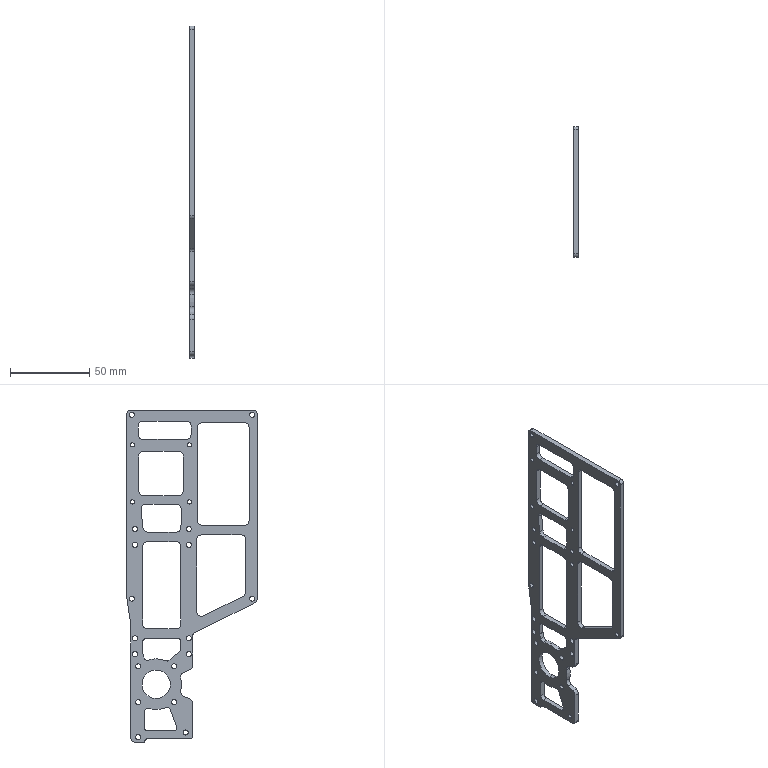Part | SolidWorks | features ICE 4, Fillet 3, Extrusion 1 | 1 solid | 146 faces | box 3 x 82 x 209.4 mm | volume 18688 mm3 | cylinder 100 | plane 46 | commonest cylinder face diameters 3.2 x36 6 x29 4 x21 2.65 x8 32 x4 18 x2